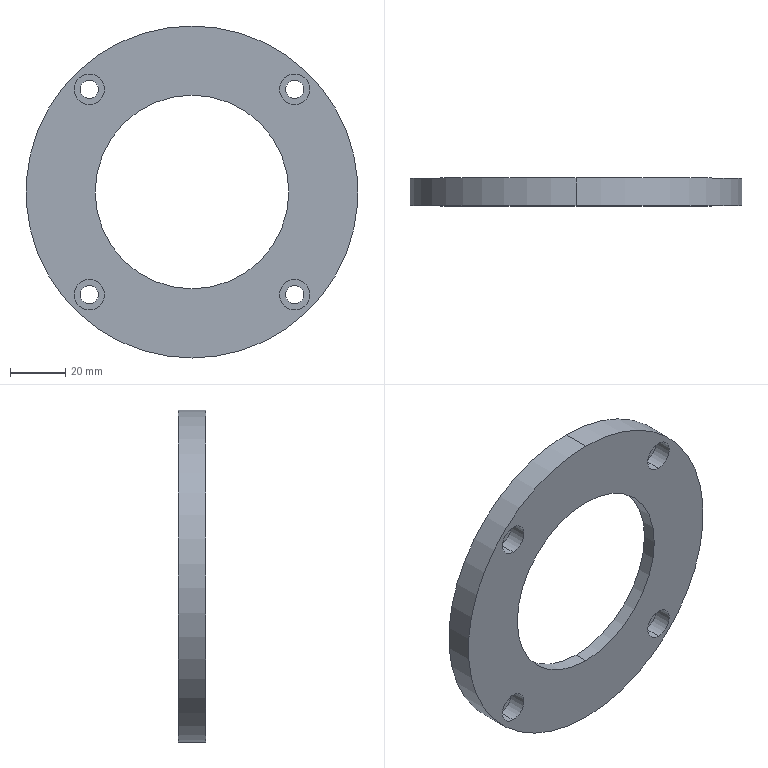Part | STEP file | 0229_208_Holder | 1 solid | 29 faces | box 120 x 10 x 120 mm | volume 60495 mm3 | cylinder 22 | plane 7 | commonest cylinder face diameters 6.6 x8 11 x8 70 x2 88 x2 120 x2